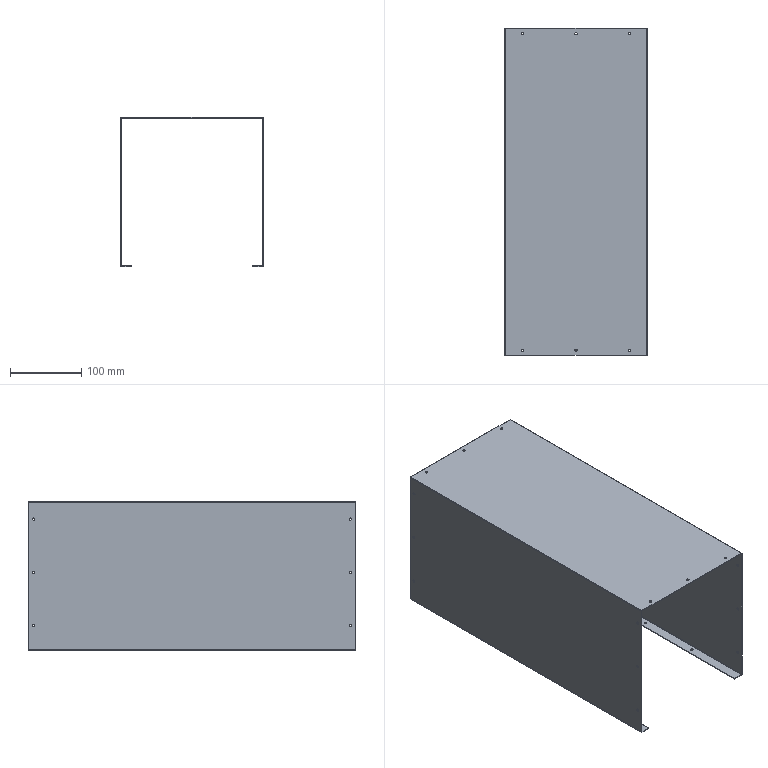Part | STEP file | TL42B-88D-1-plate heat exchanger 1 | 1 solid | 74 faces | box 200 x 460 x 210 mm | volume 296477 mm3 | cylinder 60 | plane 14 | commonest cylinder face diameters 3.2 x52 0.2 x4 2.2 x4